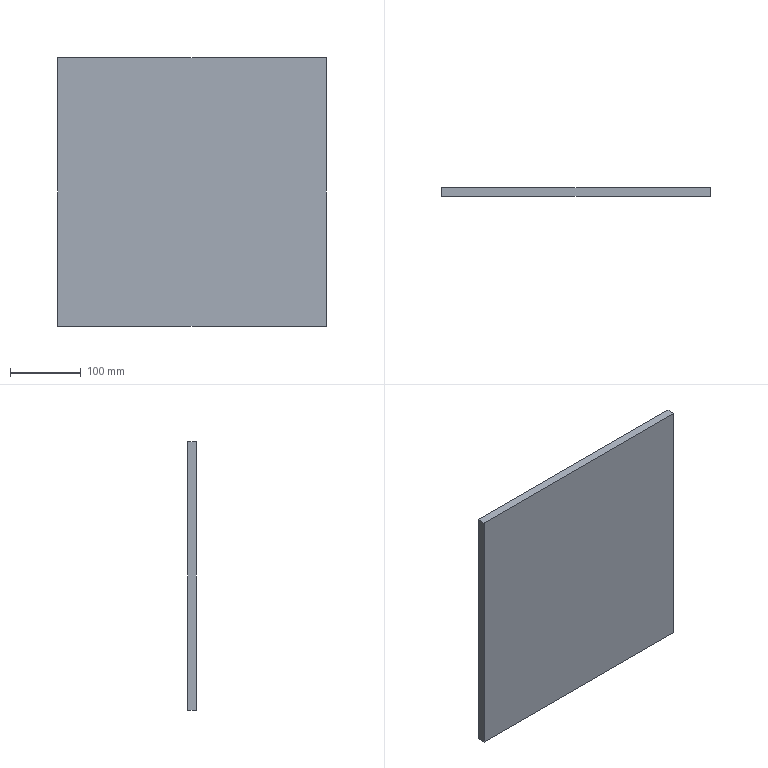Part | STEP file | Produce dryer line heating fan-SIROCCOFAN-3KW-102 | 1 solid | 6 faces | box 380 x 12 x 380 mm | volume 1732800 mm3 | plane 6
STEP:
#1=CARTESIAN_POINT('',(-190.,0.,-190.));
#2=VERTEX_POINT('',#1);
#3=CARTESIAN_POINT('',(-190.,0.,190.));
#4=VERTEX_POINT('',#3);
#5=CARTESIAN_POINT('',(-190.,0.,-190.));
#6=DIRECTION('',(0.,0.,1.));
#7=VECTOR('',#6,1000.);
#8=LINE('',#5,#7);
#9=EDGE_CURVE('',#2,#4,#8,.T.);
#10=ORIENTED_EDGE('',*,*,#9,.T.);
#11=CARTESIAN_POINT('',(-190.,12.,190.));
#12=VERTEX_POINT('',#11);
#13=CARTESIAN_POINT('',(-190.,12.,190.));
#14=DIRECTION('',(0.,-1.,0.));
#15=VECTOR('',#14,1000.);
#16=LINE('',#13,#15);
#17=EDGE_CURVE('',#12,#4,#16,.T.);
#18=ORIENTED_EDGE('',*,*,#17,.F.);
#19=CARTESIAN_POINT('',(-190.,12.,-190.));
#20=VERTEX_POINT('',#19);
#21=CARTESIAN_POINT('',(-190.,12.,-190.));
#22=DIRECTION('',(0.,0.,1.));
#23=VECTOR('',#22,1000.);
#24=LINE('',#21,#23);
#25=EDGE_CURVE('',#20,#12,#24,.T.);
#26=ORIENTED_EDGE('',*,*,#25,.F.);
#27=CARTESIAN_POINT('',(-190.,12.,-190.));
#28=DIRECTION('',(0.,-1.,0.));
#29=VECTOR('',#28,1000.);
#30=LINE('',#27,#29);
#31=EDGE_CURVE('',#20,#2,#30,.T.);
#32=ORIENTED_EDGE('',*,*,#31,.T.);
#33=EDGE_LOOP('',(#10,#18,#26,#32));
#34=FACE_OUTER_BOUND('',#33,.T.);
#35=CARTESIAN_POINT('',(-190.,12.,-190.));
#36=DIRECTION('',(1.,0.,0.));
#37=DIRECTION('',(0.,0.,-1.));
#38=AXIS2_PLACEMENT_3D('',#35,#36,#37);
#39=PLANE('',#38);
#40=ADVANCED_FACE('',(#34),#39,.F.);
#41=CARTESIAN_POINT('',(190.,0.,190.));
#42=VERTEX_POINT('',#41);
#43=CARTESIAN_POINT('',(-190.,0.,190.));
#44=DIRECTION('',(1.,0.,0.));
#45=VECTOR('',#44,1000.);
#46=LINE('',#43,#45);
#47=EDGE_CURVE('',#4,#42,#46,.T.);
#48=ORIENTED_EDGE('',*,*,#47,.T.);
#49=CARTESIAN_POINT('',(190.,12.,190.));
#50=VERTEX_POINT('',#49);
#51=CARTESIAN_POINT('',(190.,12.,190.));
#52=DIRECTION('',(0.,-1.,0.));
#53=VECTOR('',#52,1000.);
#54=LINE('',#51,#53);
#55=EDGE_CURVE('',#50,#42,#54,.T.);
#56=ORIENTED_EDGE('',*,*,#55,.F.);
#57=CARTESIAN_POINT('',(-190.,12.,190.));
#58=DIRECTION('',(1.,0.,0.));
#59=VECTOR('',#58,1000.);
#60=LINE('',#57,#59);
#61=EDGE_CURVE('',#12,#50,#60,.T.);
#62=ORIENTED_EDGE('',*,*,#61,.F.);
#63=ORIENTED_EDGE('',*,*,#17,.T.);
#64=EDGE_LOOP('',(#48,#56,#62,#63));
#65=FACE_OUTER_BOUND('',#64,.T.);
#66=CARTESIAN_POINT('',(-190.,12.,190.));
#67=DIRECTION('',(0.,0.,-1.));
#68=DIRECTION('',(-1.,0.,0.));
#69=AXIS2_PLACEMENT_3D('',#66,#67,#68);
#70=PLANE('',#69);
#71=ADVANCED_FACE('',(#65),#70,.F.);
#72=CARTESIAN_POINT('',(190.,0.,-190.));
#73=VERTEX_POINT('',#72);
#74=CARTESIAN_POINT('',(190.,0.,-190.));
#75=DIRECTION('',(0.,0.,-1.));
#76=VECTOR('',#75,1000.);
#77=LINE('',#74,#76);
#78=EDGE_CURVE('',#42,#73,#77,.T.);
#79=ORIENTED_EDGE('',*,*,#78,.T.);
#80=CARTESIAN_POINT('',(190.,12.,-190.));
#81=VERTEX_POINT('',#80);
#82=CARTESIAN_POINT('',(190.,12.,-190.));
#83=DIRECTION('',(0.,-1.,0.));
#84=VECTOR('',#83,1000.);
#85=LINE('',#82,#84);
#86=EDGE_CURVE('',#81,#73,#85,.T.);
#87=ORIENTED_EDGE('',*,*,#86,.F.);
#88=CARTESIAN_POINT('',(190.,12.,-190.));
#89=DIRECTION('',(0.,0.,-1.));
#90=VECTOR('',#89,1000.);
#91=LINE('',#88,#90);
#92=EDGE_CURVE('',#50,#81,#91,.T.);
#93=ORIENTED_EDGE('',*,*,#92,.F.);
#94=ORIENTED_EDGE('',*,*,#55,.T.);
#95=EDGE_LOOP('',(#79,#87,#93,#94));
#96=FACE_OUTER_BOUND('',#95,.T.);
#97=CARTESIAN_POINT('',(190.,12.,-190.));
#98=DIRECTION('',(-1.,0.,0.));
#99=DIRECTION('',(0.,0.,1.));
#100=AXIS2_PLACEMENT_3D('',#97,#98,#99);
#101=PLANE('',#100);
#102=ADVANCED_FACE('',(#96),#101,.F.);
#103=CARTESIAN_POINT('',(-190.,0.,-190.));
#104=DIRECTION('',(-1.,0.,0.));
#105=VECTOR('',#104,1000.);
#106=LINE('',#103,#105);
#107=EDGE_CURVE('',#73,#2,#106,.T.);
#108=ORIENTED_EDGE('',*,*,#107,.T.);
#109=ORIENTED_EDGE('',*,*,#31,.F.);
#110=CARTESIAN_POINT('',(-190.,12.,-190.));
#111=DIRECTION('',(-1.,0.,0.));
#112=VECTOR('',#111,1000.);
#113=LINE('',#110,#112);
#114=EDGE_CURVE('',#81,#20,#113,.T.);
#115=ORIENTED_EDGE('',*,*,#114,.F.);
#116=ORIENTED_EDGE('',*,*,#86,.T.);
#117=EDGE_LOOP('',(#108,#109,#115,#116));
#118=FACE_OUTER_BOUND('',#117,.T.);
#119=CARTESIAN_POINT('',(-190.,12.,-190.));
#120=DIRECTION('',(0.,0.,1.));
#121=DIRECTION('',(1.,0.,0.));
#122=AXIS2_PLACEMENT_3D('',#119,#120,#121);
#123=PLANE('',#122);
#124=ADVANCED_FACE('',(#118),#123,.F.);
#125=ORIENTED_EDGE('',*,*,#25,.T.);
#126=ORIENTED_EDGE('',*,*,#61,.T.);
#127=ORIENTED_EDGE('',*,*,#92,.T.);
#128=ORIENTED_EDGE('',*,*,#114,.T.);
#129=EDGE_LOOP('',(#125,#126,#127,#128));
#130=FACE_OUTER_BOUND('',#129,.T.);
#131=CARTESIAN_POINT('',(-190.,12.,190.));
#132=DIRECTION('',(0.,1.,0.));
#133=DIRECTION('',(0.,0.,1.));
#134=AXIS2_PLACEMENT_3D('',#131,#132,#133);
#135=PLANE('',#134);
#136=ADVANCED_FACE('',(#130),#135,.T.);
#137=ORIENTED_EDGE('',*,*,#9,.F.);
#138=ORIENTED_EDGE('',*,*,#107,.F.);
#139=ORIENTED_EDGE('',*,*,#78,.F.);
#140=ORIENTED_EDGE('',*,*,#47,.F.);
#141=EDGE_LOOP('',(#137,#138,#139,#140));
#142=FACE_OUTER_BOUND('',#141,.T.);
#143=CARTESIAN_POINT('',(-190.,0.,190.));
#144=DIRECTION('',(0.,1.,0.));
#145=DIRECTION('',(0.,0.,1.));
#146=AXIS2_PLACEMENT_3D('',#143,#144,#145);
#147=PLANE('',#146);
#148=ADVANCED_FACE('',(#142),#147,.F.);
#149=CLOSED_SHELL('',(#40,#71,#102,#124,#136,#148));
#150=MANIFOLD_SOLID_BREP('',#149);
#151=CARTESIAN_POINT('',(0.,0.,0.));
#152=DIRECTION('',(0.,0.,1.));
#153=DIRECTION('',(1.,0.,0.));
#154=AXIS2_PLACEMENT_3D('',#151,#152,#153);
#155=(LENGTH_UNIT()NAMED_UNIT(*)SI_UNIT(.MILLI.,.METRE.));
#156=UNCERTAINTY_MEASURE_WITH_UNIT(LENGTH_MEASURE(0.00001),#155,'','');
#157=(NAMED_UNIT(*)PLANE_ANGLE_UNIT()SI_UNIT($,.RADIAN.));
#158=(NAMED_UNIT(*)SI_UNIT($,.STERADIAN.)SOLID_ANGLE_UNIT());
#159=(GEOMETRIC_REPRESENTATION_CONTEXT(3)GLOBAL_UNCERTAINTY_ASSIGNED_CONTEXT((#156))GLOBAL_UNIT_ASSIGNED_CONTEXT((#155,#157,#158))REPRESENTATION_CONTEXT('',''));
#160=ADVANCED_BREP_SHAPE_REPRESENTATION('',(#150,#154),#159);